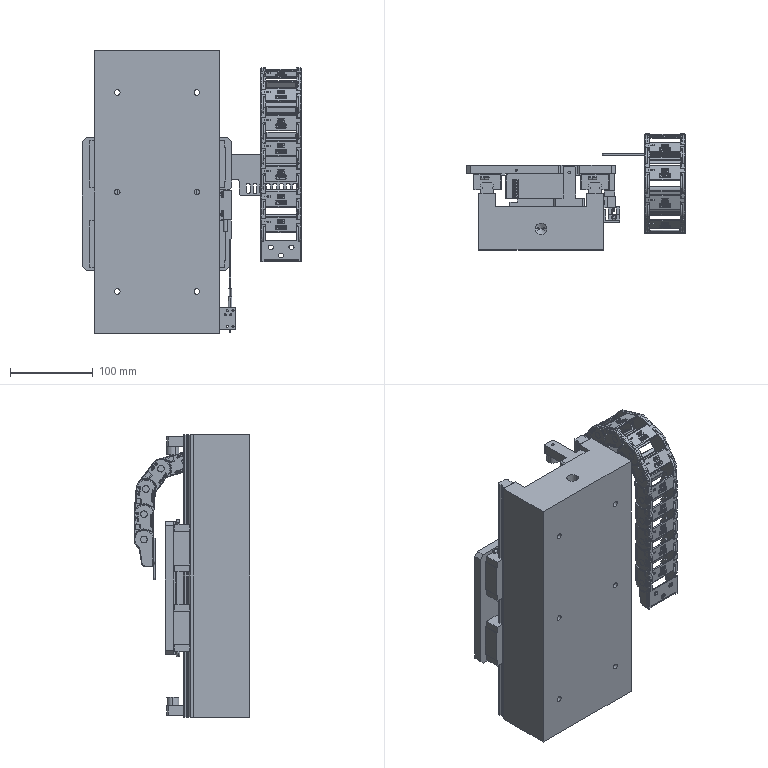Part | NX | features BREP 46 | 52 solids | 9074 faces | volume 3906926 mm3 | plane 5011 | cylinder 2114 | spline 1538 | torus 239 | cone 172 | commonest cylinder face diameters 2 x312 1 x209 0.055 x132 4.5 x124 3.3 x106 8 x106